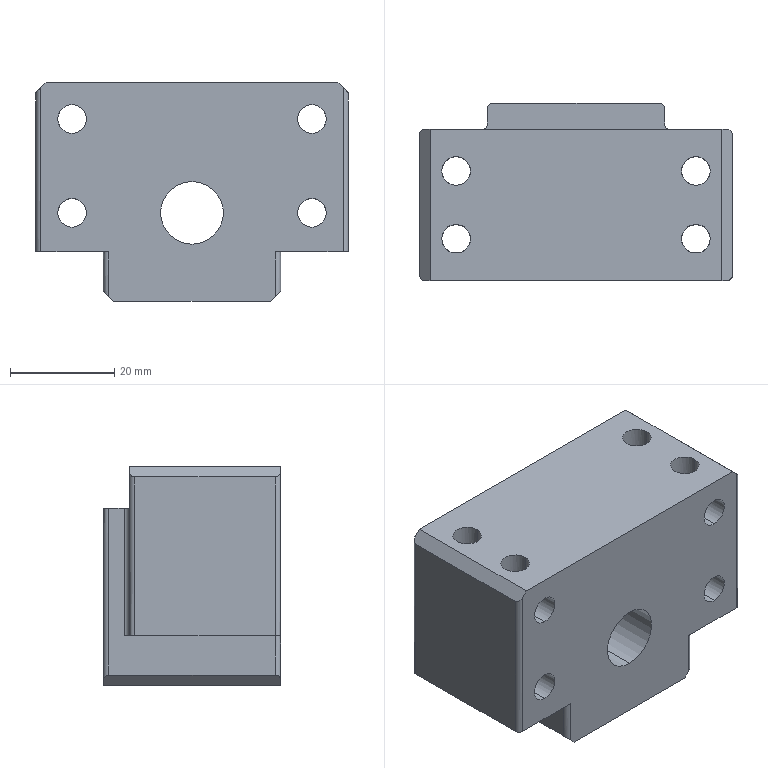Part | SolidWorks | features BaseBody 1 | 1 solid | 108 faces | box 60 x 34 x 42 mm | volume 62128 mm3 | cylinder 76 | plane 24 | cone 8 | commonest cylinder face diameters 5.5 x48 2 x10 6 x8 11 x8 12 x2